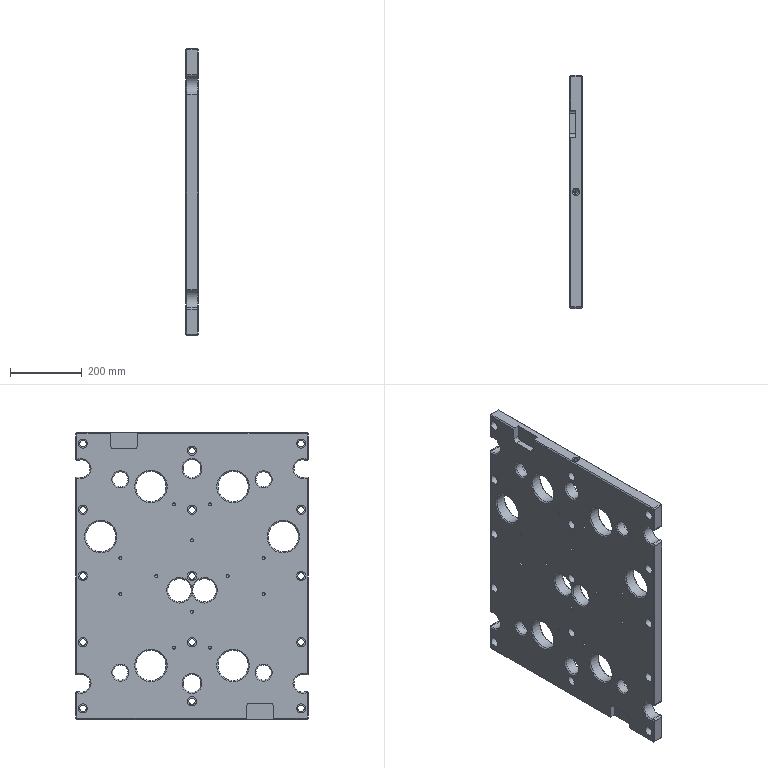Part | STEP file | solid 17 | 1 solid | 227 faces | box 35 x 650 x 800 mm | volume 15784723 mm3 | plane 81 | cylinder 78 | cone 68 | commonest cylinder face diameters 18 x15 26 x15 8.5 x12 10 x8 50 x6 85 x6